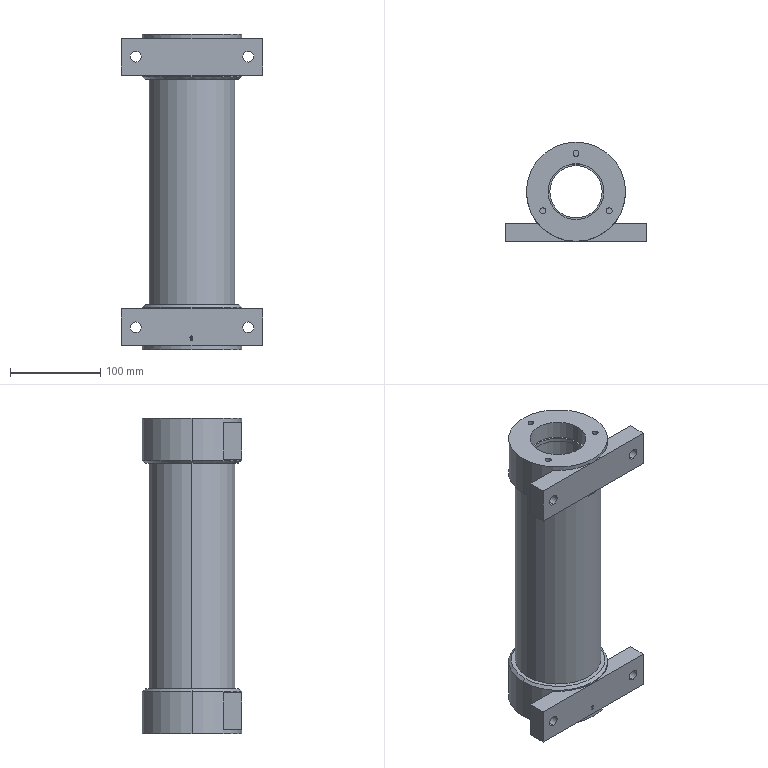Part | SolidWorks | features ICE 8, Chamfer 1, Extrusion 1 | 1 solid | 190 faces | box 157 x 110 x 350 mm | volume 1792714 mm3 | plane 123 | cylinder 34 | spline 29 | cone 4 | commonest cylinder face diameters 6.5 x12 12 x8 62 x4 110 x4 58 x2 72 x2